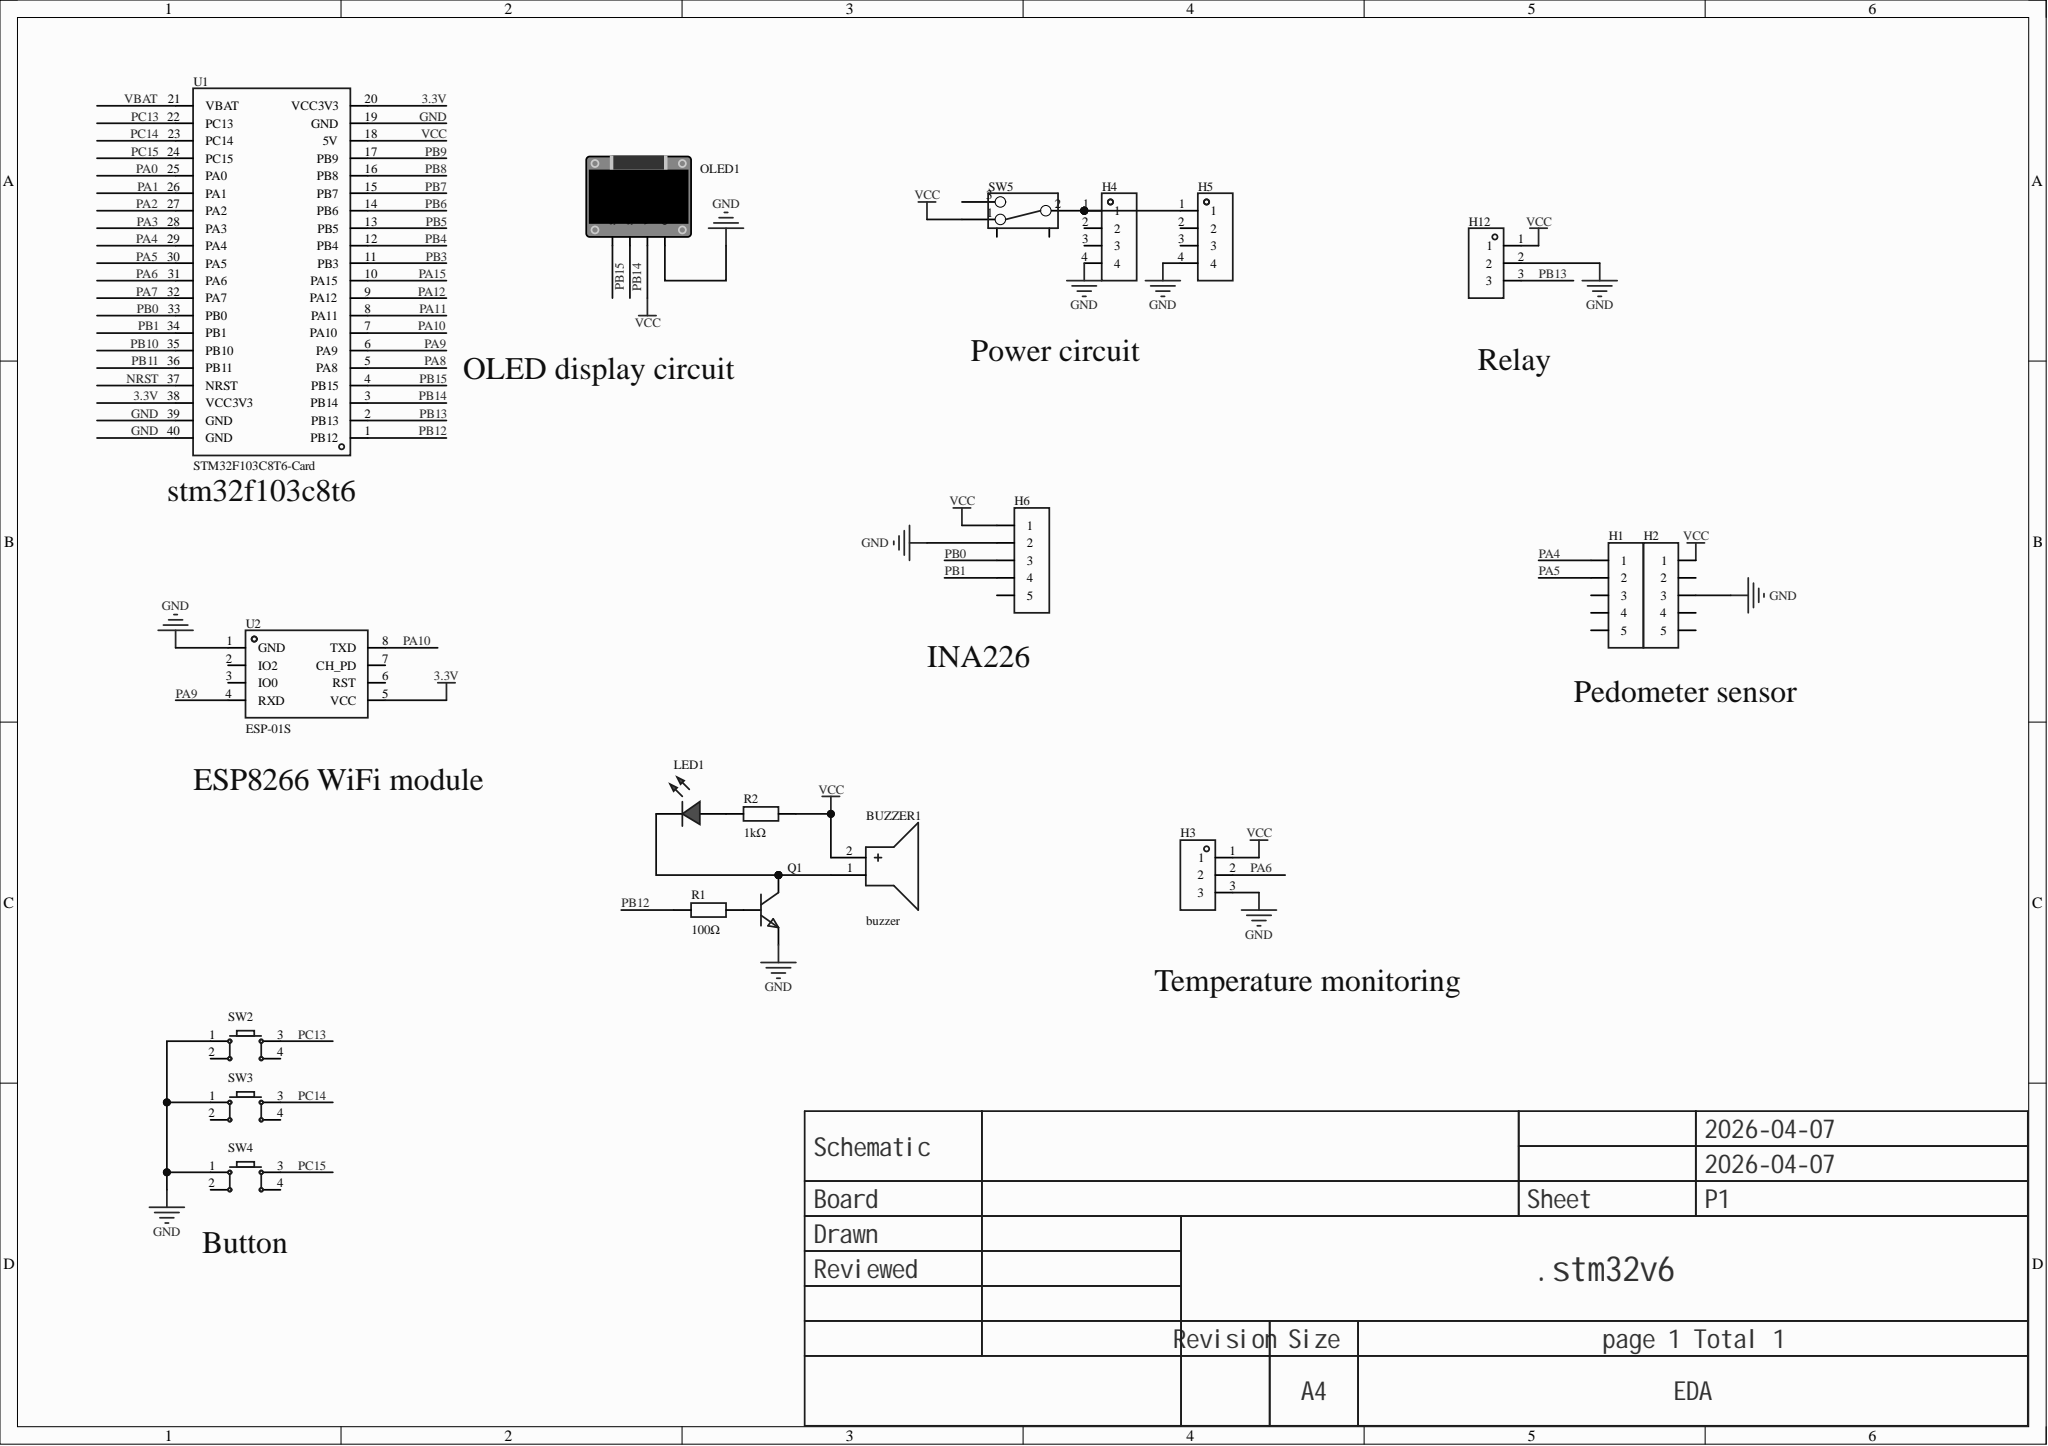Circuit board | Altium Designer | 19 parts | 21 nets
Bill of materials:
Comment,Description,Designator,Footprint,LibRef,Quantity
"buzzer","","BUZZER1","BUZ-TH_BD12.0-P6.00-D0.9-RD","buzzer","1"
"","","H1, H2, H6","HDR-TH_5P-P2.54-V-F","HDR-F_2.54_1x5P","3"
"","","H3, H12","HDR-TH_3P-P2.54-V-F","HDR-F_2.54_1x3P","2"
"","","H4, H5","HDR-TH_4P-P2.54-V-F","HDR-F_2.54_1x4P","2"
"","","LED1","LED_TH-3mm","LED_TH-R_3mm","1"
"","","OLED1","0.96OLED_4P","0.96OLED模块_4P","1"
"","","Q1","S8050_TO_92","S8050_TO_NPN","1"
"100Ω","","R1","Res_1/8W","Res_AXIAL-1/8W","1"
"1kΩ","","R2","Res_1/8W","Res_AXIAL-1/8W","1"
"","","SW2, SW3, SW4","SW-TH_4P-L6.0-W6.0-P4.50-LS6.5","Key_TH_6x6x6","3"
"","","SW5","拨动开关","拨动开关_正","1"
"STM32F103C8T6-Card","","U1","CONN-TH_L53.3-W22.9_STM32F103C8T6-CARD","STM32F103C8T6-Card","1"
"ESP-01S","","U2","WIFIM-TH_ESP-01S","ESP-01S_C111009","1"
Netlist (Protel format):
[
BUZZER1
BUZ-TH_BD12.0-P6.00-D0.9-RD
buzzer



]
[
H1
HDR-TH_5P-P2.54-V-F




]
[
H2
HDR-TH_5P-P2.54-V-F




]
[
H3
HDR-TH_3P-P2.54-V-F




]
[
H4
HDR-TH_4P-P2.54-V-F




]
[
H5
HDR-TH_4P-P2.54-V-F




]
[
H6
HDR-TH_5P-P2.54-V-F




]
[
H12
HDR-TH_3P-P2.54-V-F




]
[
LED1
LED_TH-3mm




]
[
OLED1
0.96OLED_4P




]
[
Q1
S8050_TO_92




]
[
R1
Res_1/8W
100Ω



]
[
R2
Res_1/8W
1kΩ



]
[
SW2
SW-TH_4P-L6.0-W6.0-P4.50-LS6.5




]
[
SW3
SW-TH_4P-L6.0-W6.0-P4.50-LS6.5




]
[
SW4
SW-TH_4P-L6.0-W6.0-P4.50-LS6.5




]
[
SW5
拨动开关




]
[
U1
CONN-TH_L53.3-W22.9_STM32F103C8T6-CARD
STM32F103C8T6-Card



]
[
U2
WIFIM-TH_ESP-01S
ESP-01S



]
(
VCC
BUZZER1-2
H2-1
H3-1
H6-1
H12-1
OLED1-2
R2-2
SW5-1
U1-18
)
(
PC15
SW4-3
U1-24
)
(
PC14
SW3-3
U1-23
)
(
PC13
SW2-3
U1-22
)
(
PB15
OLED1-4
U1-4
)
(
PB14
OLED1-3
U1-3
)
(
PB13
H12-3
U1-2
)
(
PB12
R1-1
U1-1
)
(
PB1
H6-4
U1-34
)
(
PB0
H6-3
U1-33
)
(
PA10
U1-7
U2-8
)
(
PA9
U1-6
U2-4
)
(
PA6
H3-2
U1-31
)
(
PA5
H1-2
U1-30
)
(
PA4
H1-1
U1-29
)
(
NetQ1_2
Q1-2
R1-2
)
(
NetLED1_1
LED1-1
R2-1
)
(
NetH4_1
H4-1
H5-1
SW5-2
)
(
NetBUZZER1_1
BUZZER1-1
LED1-2
Q1-3
)
(
GND
H2-3
H3-3
H4-4
H5-4
H6-2
H12-2
OLED1-1
Q1-1
SW2-1
SW3-1
SW4-1
U1-19
U1-39
U1-40
U2-1
)
(
3.3V
U1-20
U1-38
U2-5
)